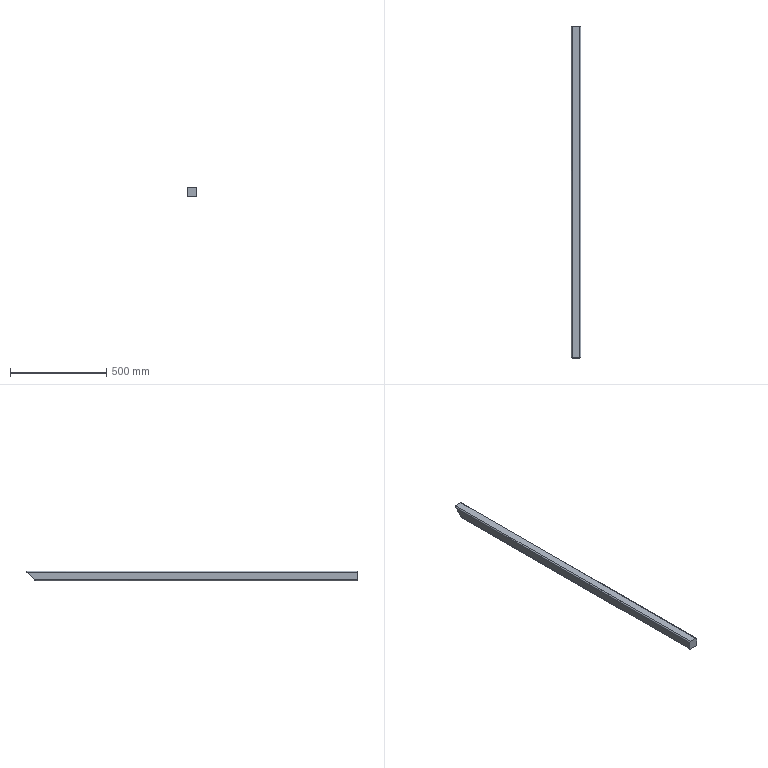Part | SolidWorks | features ICE 4, Extrusion 1 | 1 solid | 19 faces | box 50 x 1725 x 50 mm | volume 1494916 mm3 | plane 11 | cylinder 8 | commonest cylinder face diameters 2 x4 12 x4
STEP:
#1=CARTESIAN_POINT('',(-19.,1770.,7.278));
#2=VERTEX_POINT('',#1);
#3=CARTESIAN_POINT('',(-19.,60.,7.278));
#4=VERTEX_POINT('',#3);
#5=CARTESIAN_POINT('',(-19.,1775.,7.278));
#6=DIRECTION('',(0.,-1.,0.));
#7=VECTOR('',#6,1000.);
#8=LINE('',#5,#7);
#9=EDGE_CURVE('',#2,#4,#8,.T.);
#10=ORIENTED_EDGE('',*,*,#9,.T.);
#11=CARTESIAN_POINT('',(-20.,60.,6.278));
#12=VERTEX_POINT('',#11);
#13=CARTESIAN_POINT('',(-19.,60.,6.278));
#14=DIRECTION('',(0.,-1.,0.));
#15=DIRECTION('',(0.,0.,-1.));
#16=AXIS2_PLACEMENT_3D('',#13,#14,#15);
#17=CIRCLE('',#16,1.);
#18=EDGE_CURVE('',#4,#12,#17,.T.);
#19=ORIENTED_EDGE('',*,*,#18,.T.);
#20=CARTESIAN_POINT('',(-20.,1769.,6.278));
#21=VERTEX_POINT('',#20);
#22=CARTESIAN_POINT('',(-20.,1775.,6.278));
#23=DIRECTION('',(0.,-1.,0.));
#24=VECTOR('',#23,1000.);
#25=LINE('',#22,#24);
#26=EDGE_CURVE('',#21,#12,#25,.T.);
#27=ORIENTED_EDGE('',*,*,#26,.F.);
#28=CARTESIAN_POINT('',(-19.,1770.,7.278));
#29=CARTESIAN_POINT('',(-19.586,1770.,7.278));
#30=CARTESIAN_POINT('',(-20.,1769.586,6.864));
#31=CARTESIAN_POINT('',(-20.,1769.,6.278));
#32=(BOUNDED_CURVE()B_SPLINE_CURVE(3,(#28,#29,#30,#31),.UNSPECIFIED.,.F.,.F.)B_SPLINE_CURVE_WITH_KNOTS((4,4),(3.142,4.712),.UNSPECIFIED.)CURVE()GEOMETRIC_REPRESENTATION_ITEM()RATIONAL_B_SPLINE_CURVE((1.,0.8047,0.8047,1.))REPRESENTATION_ITEM(''));
#33=EDGE_CURVE('',#2,#21,#32,.T.);
#34=ORIENTED_EDGE('',*,*,#33,.F.);
#35=EDGE_LOOP('',(#10,#19,#27,#34));
#36=FACE_OUTER_BOUND('',#35,.T.);
#37=CARTESIAN_POINT('',(-19.,1775.,6.278));
#38=DIRECTION('',(0.,-1.,0.));
#39=DIRECTION('',(0.,0.,-1.));
#40=AXIS2_PLACEMENT_3D('',#37,#38,#39);
#41=CYLINDRICAL_SURFACE('',#40,1.);
#42=ADVANCED_FACE('',(#36),#41,.F.);
#43=CARTESIAN_POINT('',(19.,1770.,7.278));
#44=VERTEX_POINT('',#43);
#45=CARTESIAN_POINT('',(19.,60.,7.278));
#46=VERTEX_POINT('',#45);
#47=CARTESIAN_POINT('',(19.,1775.,7.278));
#48=DIRECTION('',(0.,-1.,0.));
#49=VECTOR('',#48,1000.);
#50=LINE('',#47,#49);
#51=EDGE_CURVE('',#44,#46,#50,.T.);
#52=ORIENTED_EDGE('',*,*,#51,.T.);
#53=CARTESIAN_POINT('',(-19.,60.,7.278));
#54=DIRECTION('',(-1.,0.,0.));
#55=VECTOR('',#54,1000.);
#56=LINE('',#53,#55);
#57=EDGE_CURVE('',#46,#4,#56,.T.);
#58=ORIENTED_EDGE('',*,*,#57,.T.);
#59=ORIENTED_EDGE('',*,*,#9,.F.);
#60=CARTESIAN_POINT('',(-19.,1770.,7.278));
#61=DIRECTION('',(-1.,0.,0.));
#62=VECTOR('',#61,1000.);
#63=LINE('',#60,#62);
#64=EDGE_CURVE('',#44,#2,#63,.T.);
#65=ORIENTED_EDGE('',*,*,#64,.F.);
#66=EDGE_LOOP('',(#52,#58,#59,#65));
#67=FACE_OUTER_BOUND('',#66,.T.);
#68=CARTESIAN_POINT('',(-19.,1775.,7.278));
#69=DIRECTION('',(0.,0.,-1.));
#70=DIRECTION('',(-1.,0.,0.));
#71=AXIS2_PLACEMENT_3D('',#68,#69,#70);
#72=PLANE('',#71);
#73=ADVANCED_FACE('',(#67),#72,.T.);
#74=CARTESIAN_POINT('',(20.,1769.,6.278));
#75=VERTEX_POINT('',#74);
#76=CARTESIAN_POINT('',(20.,60.,6.278));
#77=VERTEX_POINT('',#76);
#78=CARTESIAN_POINT('',(20.,1775.,6.278));
#79=DIRECTION('',(0.,-1.,0.));
#80=VECTOR('',#79,1000.);
#81=LINE('',#78,#80);
#82=EDGE_CURVE('',#75,#77,#81,.T.);
#83=ORIENTED_EDGE('',*,*,#82,.T.);
#84=CARTESIAN_POINT('',(19.,60.,6.278));
#85=DIRECTION('',(0.,-1.,0.));
#86=DIRECTION('',(0.,0.,-1.));
#87=AXIS2_PLACEMENT_3D('',#84,#85,#86);
#88=CIRCLE('',#87,1.);
#89=EDGE_CURVE('',#77,#46,#88,.T.);
#90=ORIENTED_EDGE('',*,*,#89,.T.);
#91=ORIENTED_EDGE('',*,*,#51,.F.);
#92=CARTESIAN_POINT('',(20.,1769.,6.278));
#93=CARTESIAN_POINT('',(20.,1769.586,6.864));
#94=CARTESIAN_POINT('',(19.586,1770.,7.278));
#95=CARTESIAN_POINT('',(19.,1770.,7.278));
#96=(BOUNDED_CURVE()B_SPLINE_CURVE(3,(#92,#93,#94,#95),.UNSPECIFIED.,.F.,.F.)B_SPLINE_CURVE_WITH_KNOTS((4,4),(1.571,3.142),.UNSPECIFIED.)CURVE()GEOMETRIC_REPRESENTATION_ITEM()RATIONAL_B_SPLINE_CURVE((1.,0.8047,0.8047,1.))REPRESENTATION_ITEM(''));
#97=EDGE_CURVE('',#75,#44,#96,.T.);
#98=ORIENTED_EDGE('',*,*,#97,.F.);
#99=EDGE_LOOP('',(#83,#90,#91,#98));
#100=FACE_OUTER_BOUND('',#99,.T.);
#101=CARTESIAN_POINT('',(19.,1775.,6.278));
#102=DIRECTION('',(0.,-1.,0.));
#103=DIRECTION('',(0.,0.,-1.));
#104=AXIS2_PLACEMENT_3D('',#101,#102,#103);
#105=CYLINDRICAL_SURFACE('',#104,1.);
#106=ADVANCED_FACE('',(#100),#105,.F.);
#107=CARTESIAN_POINT('',(20.,1731.,-31.722));
#108=VERTEX_POINT('',#107);
#109=CARTESIAN_POINT('',(20.,60.,-31.722));
#110=VERTEX_POINT('',#109);
#111=CARTESIAN_POINT('',(20.,1775.,-31.722));
#112=DIRECTION('',(0.,-1.,0.));
#113=VECTOR('',#112,1000.);
#114=LINE('',#111,#113);
#115=EDGE_CURVE('',#108,#110,#114,.T.);
#116=ORIENTED_EDGE('',*,*,#115,.T.);
#117=CARTESIAN_POINT('',(20.,60.,6.278));
#118=DIRECTION('',(0.,0.,1.));
#119=VECTOR('',#118,1000.);
#120=LINE('',#117,#119);
#121=EDGE_CURVE('',#110,#77,#120,.T.);
#122=ORIENTED_EDGE('',*,*,#121,.T.);
#123=ORIENTED_EDGE('',*,*,#82,.F.);
#124=CARTESIAN_POINT('',(20.,1772.,9.278));
#125=DIRECTION('',(0.,0.7071,0.7071));
#126=VECTOR('',#125,1000.);
#127=LINE('',#124,#126);
#128=EDGE_CURVE('',#108,#75,#127,.T.);
#129=ORIENTED_EDGE('',*,*,#128,.F.);
#130=EDGE_LOOP('',(#116,#122,#123,#129));
#131=FACE_OUTER_BOUND('',#130,.T.);
#132=CARTESIAN_POINT('',(20.,1775.,6.278));
#133=DIRECTION('',(-1.,0.,0.));
#134=DIRECTION('',(0.,0.,1.));
#135=AXIS2_PLACEMENT_3D('',#132,#133,#134);
#136=PLANE('',#135);
#137=ADVANCED_FACE('',(#131),#136,.T.);
#138=CARTESIAN_POINT('',(19.,1730.,-32.722));
#139=VERTEX_POINT('',#138);
#140=CARTESIAN_POINT('',(19.,60.,-32.722));
#141=VERTEX_POINT('',#140);
#142=CARTESIAN_POINT('',(19.,1775.,-32.722));
#143=DIRECTION('',(0.,-1.,0.));
#144=VECTOR('',#143,1000.);
#145=LINE('',#142,#144);
#146=EDGE_CURVE('',#139,#141,#145,.T.);
#147=ORIENTED_EDGE('',*,*,#146,.T.);
#148=CARTESIAN_POINT('',(19.,60.,-31.722));
#149=DIRECTION('',(0.,-1.,0.));
#150=DIRECTION('',(0.,0.,-1.));
#151=AXIS2_PLACEMENT_3D('',#148,#149,#150);
#152=CIRCLE('',#151,1.);
#153=EDGE_CURVE('',#141,#110,#152,.T.);
#154=ORIENTED_EDGE('',*,*,#153,.T.);
#155=ORIENTED_EDGE('',*,*,#115,.F.);
#156=CARTESIAN_POINT('',(19.,1730.,-32.722));
#157=CARTESIAN_POINT('',(19.586,1730.,-32.722));
#158=CARTESIAN_POINT('',(20.,1730.414,-32.308));
#159=CARTESIAN_POINT('',(20.,1731.,-31.722));
#160=(BOUNDED_CURVE()B_SPLINE_CURVE(3,(#156,#157,#158,#159),.UNSPECIFIED.,.F.,.F.)B_SPLINE_CURVE_WITH_KNOTS((4,4),(0.,1.571),.UNSPECIFIED.)CURVE()GEOMETRIC_REPRESENTATION_ITEM()RATIONAL_B_SPLINE_CURVE((1.,0.8047,0.8047,1.))REPRESENTATION_ITEM(''));
#161=EDGE_CURVE('',#139,#108,#160,.T.);
#162=ORIENTED_EDGE('',*,*,#161,.F.);
#163=EDGE_LOOP('',(#147,#154,#155,#162));
#164=FACE_OUTER_BOUND('',#163,.T.);
#165=CARTESIAN_POINT('',(19.,1775.,-31.722));
#166=DIRECTION('',(0.,-1.,0.));
#167=DIRECTION('',(0.,0.,-1.));
#168=AXIS2_PLACEMENT_3D('',#165,#166,#167);
#169=CYLINDRICAL_SURFACE('',#168,1.);
#170=ADVANCED_FACE('',(#164),#169,.F.);
#171=CARTESIAN_POINT('',(-19.,1730.,-32.722));
#172=VERTEX_POINT('',#171);
#173=CARTESIAN_POINT('',(-19.,60.,-32.722));
#174=VERTEX_POINT('',#173);
#175=CARTESIAN_POINT('',(-19.,1775.,-32.722));
#176=DIRECTION('',(0.,-1.,0.));
#177=VECTOR('',#176,1000.);
#178=LINE('',#175,#177);
#179=EDGE_CURVE('',#172,#174,#178,.T.);
#180=ORIENTED_EDGE('',*,*,#179,.T.);
#181=CARTESIAN_POINT('',(-19.,60.,-32.722));
#182=DIRECTION('',(1.,0.,0.));
#183=VECTOR('',#182,1000.);
#184=LINE('',#181,#183);
#185=EDGE_CURVE('',#174,#141,#184,.T.);
#186=ORIENTED_EDGE('',*,*,#185,.T.);
#187=ORIENTED_EDGE('',*,*,#146,.F.);
#188=CARTESIAN_POINT('',(-19.,1730.,-32.722));
#189=DIRECTION('',(1.,0.,0.));
#190=VECTOR('',#189,1000.);
#191=LINE('',#188,#190);
#192=EDGE_CURVE('',#172,#139,#191,.T.);
#193=ORIENTED_EDGE('',*,*,#192,.F.);
#194=EDGE_LOOP('',(#180,#186,#187,#193));
#195=FACE_OUTER_BOUND('',#194,.T.);
#196=CARTESIAN_POINT('',(-19.,1775.,-32.722));
#197=DIRECTION('',(0.,0.,1.));
#198=DIRECTION('',(1.,0.,0.));
#199=AXIS2_PLACEMENT_3D('',#196,#197,#198);
#200=PLANE('',#199);
#201=ADVANCED_FACE('',(#195),#200,.T.);
#202=CARTESIAN_POINT('',(-20.,1731.,-31.722));
#203=VERTEX_POINT('',#202);
#204=CARTESIAN_POINT('',(-20.,60.,-31.722));
#205=VERTEX_POINT('',#204);
#206=CARTESIAN_POINT('',(-20.,1775.,-31.722));
#207=DIRECTION('',(0.,-1.,0.));
#208=VECTOR('',#207,1000.);
#209=LINE('',#206,#208);
#210=EDGE_CURVE('',#203,#205,#209,.T.);
#211=ORIENTED_EDGE('',*,*,#210,.T.);
#212=CARTESIAN_POINT('',(-19.,60.,-31.722));
#213=DIRECTION('',(0.,-1.,0.));
#214=DIRECTION('',(0.,0.,-1.));
#215=AXIS2_PLACEMENT_3D('',#212,#213,#214);
#216=CIRCLE('',#215,1.);
#217=EDGE_CURVE('',#205,#174,#216,.T.);
#218=ORIENTED_EDGE('',*,*,#217,.T.);
#219=ORIENTED_EDGE('',*,*,#179,.F.);
#220=CARTESIAN_POINT('',(-20.,1731.,-31.722));
#221=CARTESIAN_POINT('',(-20.,1730.414,-32.308));
#222=CARTESIAN_POINT('',(-19.586,1730.,-32.722));
#223=CARTESIAN_POINT('',(-19.,1730.,-32.722));
#224=(BOUNDED_CURVE()B_SPLINE_CURVE(3,(#220,#221,#222,#223),.UNSPECIFIED.,.F.,.F.)B_SPLINE_CURVE_WITH_KNOTS((4,4),(4.712,6.283),.UNSPECIFIED.)CURVE()GEOMETRIC_REPRESENTATION_ITEM()RATIONAL_B_SPLINE_CURVE((1.,0.8047,0.8047,1.))REPRESENTATION_ITEM(''));
#225=EDGE_CURVE('',#203,#172,#224,.T.);
#226=ORIENTED_EDGE('',*,*,#225,.F.);
#227=EDGE_LOOP('',(#211,#218,#219,#226));
#228=FACE_OUTER_BOUND('',#227,.T.);
#229=CARTESIAN_POINT('',(-19.,1775.,-31.722));
#230=DIRECTION('',(0.,-1.,0.));
#231=DIRECTION('',(0.,0.,-1.));
#232=AXIS2_PLACEMENT_3D('',#229,#230,#231);
#233=CYLINDRICAL_SURFACE('',#232,1.);
#234=ADVANCED_FACE('',(#228),#233,.F.);
#235=ORIENTED_EDGE('',*,*,#26,.T.);
#236=CARTESIAN_POINT('',(-20.,60.,6.278));
#237=DIRECTION('',(0.,0.,-1.));
#238=VECTOR('',#237,1000.);
#239=LINE('',#236,#238);
#240=EDGE_CURVE('',#12,#205,#239,.T.);
#241=ORIENTED_EDGE('',*,*,#240,.T.);
#242=ORIENTED_EDGE('',*,*,#210,.F.);
#243=CARTESIAN_POINT('',(-20.,1772.,9.278));
#244=DIRECTION('',(0.,-0.7071,-0.7071));
#245=VECTOR('',#244,1000.);
#246=LINE('',#243,#245);
#247=EDGE_CURVE('',#21,#203,#246,.T.);
#248=ORIENTED_EDGE('',*,*,#247,.F.);
#249=EDGE_LOOP('',(#235,#241,#242,#248));
#250=FACE_OUTER_BOUND('',#249,.T.);
#251=CARTESIAN_POINT('',(-20.,1775.,6.278));
#252=DIRECTION('',(1.,0.,0.));
#253=DIRECTION('',(0.,0.,-1.));
#254=AXIS2_PLACEMENT_3D('',#251,#252,#253);
#255=PLANE('',#254);
#256=ADVANCED_FACE('',(#250),#255,.T.);
#257=CARTESIAN_POINT('',(-25.,50.,6.278));
#258=VERTEX_POINT('',#257);
#259=CARTESIAN_POINT('',(-19.,50.,12.278));
#260=VERTEX_POINT('',#259);
#261=CARTESIAN_POINT('',(-19.,50.,6.278));
#262=DIRECTION('',(0.,1.,0.));
#263=DIRECTION('',(0.,0.,1.));
#264=AXIS2_PLACEMENT_3D('',#261,#262,#263);
#265=CIRCLE('',#264,6.);
#266=EDGE_CURVE('',#258,#260,#265,.T.);
#267=ORIENTED_EDGE('',*,*,#266,.T.);
#268=CARTESIAN_POINT('',(-19.,1775.,12.278));
#269=VERTEX_POINT('',#268);
#270=CARTESIAN_POINT('',(-19.,1775.,12.278));
#271=DIRECTION('',(0.,-1.,0.));
#272=VECTOR('',#271,1000.);
#273=LINE('',#270,#272);
#274=EDGE_CURVE('',#269,#260,#273,.T.);
#275=ORIENTED_EDGE('',*,*,#274,.F.);
#276=CARTESIAN_POINT('',(-25.,1769.,6.278));
#277=VERTEX_POINT('',#276);
#278=CARTESIAN_POINT('',(-19.,1775.,12.278));
#279=CARTESIAN_POINT('',(-22.515,1775.,12.278));
#280=CARTESIAN_POINT('',(-25.,1772.515,9.793));
#281=CARTESIAN_POINT('',(-25.,1769.,6.278));
#282=(BOUNDED_CURVE()B_SPLINE_CURVE(3,(#278,#279,#280,#281),.UNSPECIFIED.,.F.,.F.)B_SPLINE_CURVE_WITH_KNOTS((4,4),(3.142,4.712),.UNSPECIFIED.)CURVE()GEOMETRIC_REPRESENTATION_ITEM()RATIONAL_B_SPLINE_CURVE((1.,0.8047,0.8047,1.))REPRESENTATION_ITEM(''));
#283=EDGE_CURVE('',#269,#277,#282,.T.);
#284=ORIENTED_EDGE('',*,*,#283,.T.);
#285=CARTESIAN_POINT('',(-25.,1775.,6.278));
#286=DIRECTION('',(0.,-1.,0.));
#287=VECTOR('',#286,1000.);
#288=LINE('',#285,#287);
#289=EDGE_CURVE('',#277,#258,#288,.T.);
#290=ORIENTED_EDGE('',*,*,#289,.T.);
#291=EDGE_LOOP('',(#267,#275,#284,#290));
#292=FACE_OUTER_BOUND('',#291,.T.);
#293=CARTESIAN_POINT('',(-19.,1775.,6.278));
#294=DIRECTION('',(0.,-1.,0.));
#295=DIRECTION('',(0.,0.,-1.));
#296=AXIS2_PLACEMENT_3D('',#293,#294,#295);
#297=CYLINDRICAL_SURFACE('',#296,6.);
#298=ADVANCED_FACE('',(#292),#297,.T.);
#299=CARTESIAN_POINT('',(19.,50.,12.278));
#300=VERTEX_POINT('',#299);
#301=CARTESIAN_POINT('',(-19.,50.,12.278));
#302=DIRECTION('',(1.,0.,0.));
#303=VECTOR('',#302,1000.);
#304=LINE('',#301,#303);
#305=EDGE_CURVE('',#260,#300,#304,.T.);
#306=ORIENTED_EDGE('',*,*,#305,.T.);
#307=CARTESIAN_POINT('',(19.,1775.,12.278));
#308=VERTEX_POINT('',#307);
#309=CARTESIAN_POINT('',(19.,1775.,12.278));
#310=DIRECTION('',(0.,-1.,0.));
#311=VECTOR('',#310,1000.);
#312=LINE('',#309,#311);
#313=EDGE_CURVE('',#308,#300,#312,.T.);
#314=ORIENTED_EDGE('',*,*,#313,.F.);
#315=CARTESIAN_POINT('',(-19.,1775.,12.278));
#316=DIRECTION('',(1.,0.,0.));
#317=VECTOR('',#316,1000.);
#318=LINE('',#315,#317);
#319=EDGE_CURVE('',#269,#308,#318,.T.);
#320=ORIENTED_EDGE('',*,*,#319,.F.);
#321=ORIENTED_EDGE('',*,*,#274,.T.);
#322=EDGE_LOOP('',(#306,#314,#320,#321));
#323=FACE_OUTER_BOUND('',#322,.T.);
#324=CARTESIAN_POINT('',(-19.,1775.,12.278));
#325=DIRECTION('',(0.,0.,-1.));
#326=DIRECTION('',(-1.,0.,0.));
#327=AXIS2_PLACEMENT_3D('',#324,#325,#326);
#328=PLANE('',#327);
#329=ADVANCED_FACE('',(#323),#328,.F.);
#330=CARTESIAN_POINT('',(25.,50.,6.278));
#331=VERTEX_POINT('',#330);
#332=CARTESIAN_POINT('',(19.,50.,6.278));
#333=DIRECTION('',(0.,1.,0.));
#334=DIRECTION('',(0.,0.,1.));
#335=AXIS2_PLACEMENT_3D('',#332,#333,#334);
#336=CIRCLE('',#335,6.);
#337=EDGE_CURVE('',#300,#331,#336,.T.);
#338=ORIENTED_EDGE('',*,*,#337,.T.);
#339=CARTESIAN_POINT('',(25.,1769.,6.278));
#340=VERTEX_POINT('',#339);
#341=CARTESIAN_POINT('',(25.,1775.,6.278));
#342=DIRECTION('',(0.,-1.,0.));
#343=VECTOR('',#342,1000.);
#344=LINE('',#341,#343);
#345=EDGE_CURVE('',#340,#331,#344,.T.);
#346=ORIENTED_EDGE('',*,*,#345,.F.);
#347=CARTESIAN_POINT('',(25.,1769.,6.278));
#348=CARTESIAN_POINT('',(25.,1772.515,9.793));
#349=CARTESIAN_POINT('',(22.515,1775.,12.278));
#350=CARTESIAN_POINT('',(19.,1775.,12.278));
#351=(BOUNDED_CURVE()B_SPLINE_CURVE(3,(#347,#348,#349,#350),.UNSPECIFIED.,.F.,.F.)B_SPLINE_CURVE_WITH_KNOTS((4,4),(1.571,3.142),.UNSPECIFIED.)CURVE()GEOMETRIC_REPRESENTATION_ITEM()RATIONAL_B_SPLINE_CURVE((1.,0.8047,0.8047,1.))REPRESENTATION_ITEM(''));
#352=EDGE_CURVE('',#340,#308,#351,.T.);
#353=ORIENTED_EDGE('',*,*,#352,.T.);
#354=ORIENTED_EDGE('',*,*,#313,.T.);
#355=EDGE_LOOP('',(#338,#346,#353,#354));
#356=FACE_OUTER_BOUND('',#355,.T.);
#357=CARTESIAN_POINT('',(19.,1775.,6.278));
#358=DIRECTION('',(0.,-1.,0.));
#359=DIRECTION('',(0.,0.,-1.));
#360=AXIS2_PLACEMENT_3D('',#357,#358,#359);
#361=CYLINDRICAL_SURFACE('',#360,6.);
#362=ADVANCED_FACE('',(#356),#361,.T.);
#363=CARTESIAN_POINT('',(25.,50.,-31.722));
#364=VERTEX_POINT('',#363);
#365=CARTESIAN_POINT('',(25.,50.,341.265));
#366=DIRECTION('',(0.,0.,1.));
#367=VECTOR('',#366,1000.);
#368=LINE('',#365,#367);
#369=EDGE_CURVE('',#364,#331,#368,.T.);
#370=ORIENTED_EDGE('',*,*,#369,.F.);
#371=CARTESIAN_POINT('',(25.,1731.,-31.722));
#372=VERTEX_POINT('',#371);
#373=CARTESIAN_POINT('',(25.,1775.,-31.722));
#374=DIRECTION('',(0.,-1.,0.));
#375=VECTOR('',#374,1000.);
#376=LINE('',#373,#375);
#377=EDGE_CURVE('',#372,#364,#376,.T.);
#378=ORIENTED_EDGE('',*,*,#377,.F.);
#379=CARTESIAN_POINT('',(25.,1725.,-37.722));
#380=DIRECTION('',(0.,-0.7071,-0.7071));
#381=VECTOR('',#380,1000.);
#382=LINE('',#379,#381);
#383=EDGE_CURVE('',#340,#372,#382,.T.);
#384=ORIENTED_EDGE('',*,*,#383,.F.);
#385=ORIENTED_EDGE('',*,*,#345,.T.);
#386=EDGE_LOOP('',(#370,#378,#384,#385));
#387=FACE_OUTER_BOUND('',#386,.T.);
#388=CARTESIAN_POINT('',(25.,1775.,6.278));
#389=DIRECTION('',(-1.,0.,0.));
#390=DIRECTION('',(0.,0.,1.));
#391=AXIS2_PLACEMENT_3D('',#388,#389,#390);
#392=PLANE('',#391);
#393=ADVANCED_FACE('',(#387),#392,.F.);
#394=CARTESIAN_POINT('',(19.,50.,-37.722));
#395=VERTEX_POINT('',#394);
#396=CARTESIAN_POINT('',(19.,50.,-31.722));
#397=DIRECTION('',(0.,1.,0.));
#398=DIRECTION('',(0.,0.,1.));
#399=AXIS2_PLACEMENT_3D('',#396,#397,#398);
#400=CIRCLE('',#399,6.);
#401=EDGE_CURVE('',#364,#395,#400,.T.);
#402=ORIENTED_EDGE('',*,*,#401,.T.);
#403=CARTESIAN_POINT('',(19.,1725.,-37.722));
#404=VERTEX_POINT('',#403);
#405=CARTESIAN_POINT('',(19.,1775.,-37.722));
#406=DIRECTION('',(0.,-1.,0.));
#407=VECTOR('',#406,1000.);
#408=LINE('',#405,#407);
#409=EDGE_CURVE('',#404,#395,#408,.T.);
#410=ORIENTED_EDGE('',*,*,#409,.F.);
#411=CARTESIAN_POINT('',(19.,1725.,-37.722));
#412=CARTESIAN_POINT('',(22.515,1725.,-37.722));
#413=CARTESIAN_POINT('',(25.,1727.485,-35.237));
#414=CARTESIAN_POINT('',(25.,1731.,-31.722));
#415=(BOUNDED_CURVE()B_SPLINE_CURVE(3,(#411,#412,#413,#414),.UNSPECIFIED.,.F.,.F.)B_SPLINE_CURVE_WITH_KNOTS((4,4),(0.,1.571),.UNSPECIFIED.)CURVE()GEOMETRIC_REPRESENTATION_ITEM()RATIONAL_B_SPLINE_CURVE((1.,0.8047,0.8047,1.))REPRESENTATION_ITEM(''));
#416=EDGE_CURVE('',#404,#372,#415,.T.);
#417=ORIENTED_EDGE('',*,*,#416,.T.);
#418=ORIENTED_EDGE('',*,*,#377,.T.);
#419=EDGE_LOOP('',(#402,#410,#417,#418));
#420=FACE_OUTER_BOUND('',#419,.T.);
#421=CARTESIAN_POINT('',(19.,1775.,-31.722));
#422=DIRECTION('',(0.,-1.,0.));
#423=DIRECTION('',(0.,0.,-1.));
#424=AXIS2_PLACEMENT_3D('',#421,#422,#423);
#425=CYLINDRICAL_SURFACE('',#424,6.);
#426=ADVANCED_FACE('',(#420),#425,.T.);
#427=CARTESIAN_POINT('',(-19.,50.,-37.722));
#428=VERTEX_POINT('',#427);
#429=CARTESIAN_POINT('',(-19.,50.,-37.722));
#430=DIRECTION('',(-1.,0.,0.));
#431=VECTOR('',#430,1000.);
#432=LINE('',#429,#431);
#433=EDGE_CURVE('',#395,#428,#432,.T.);
#434=ORIENTED_EDGE('',*,*,#433,.T.);
#435=CARTESIAN_POINT('',(-19.,1725.,-37.722));
#436=VERTEX_POINT('',#435);
#437=CARTESIAN_POINT('',(-19.,1775.,-37.722));
#438=DIRECTION('',(0.,-1.,0.));
#439=VECTOR('',#438,1000.);
#440=LINE('',#437,#439);
#441=EDGE_CURVE('',#436,#428,#440,.T.);
#442=ORIENTED_EDGE('',*,*,#441,.F.);
#443=CARTESIAN_POINT('',(-25.,1725.,-37.722));
#444=DIRECTION('',(1.,0.,0.));
#445=VECTOR('',#444,1000.);
#446=LINE('',#443,#445);
#447=EDGE_CURVE('',#436,#404,#446,.T.);
#448=ORIENTED_EDGE('',*,*,#447,.T.);
#449=ORIENTED_EDGE('',*,*,#409,.T.);
#450=EDGE_LOOP('',(#434,#442,#448,#449));
#451=FACE_OUTER_BOUND('',#450,.T.);
#452=CARTESIAN_POINT('',(-19.,1775.,-37.722));
#453=DIRECTION('',(0.,0.,1.));
#454=DIRECTION('',(1.,0.,0.));
#455=AXIS2_PLACEMENT_3D('',#452,#453,#454);
#456=PLANE('',#455);
#457=ADVANCED_FACE('',(#451),#456,.F.);
#458=CARTESIAN_POINT('',(-25.,50.,-31.722));
#459=VERTEX_POINT('',#458);
#460=CARTESIAN_POINT('',(-19.,50.,-31.722));
#461=DIRECTION('',(0.,1.,0.));
#462=DIRECTION('',(0.,0.,1.));
#463=AXIS2_PLACEMENT_3D('',#460,#461,#462);
#464=CIRCLE('',#463,6.);
#465=EDGE_CURVE('',#428,#459,#464,.T.);
#466=ORIENTED_EDGE('',*,*,#465,.T.);
#467=CARTESIAN_POINT('',(-25.,1731.,-31.722));
#468=VERTEX_POINT('',#467);
#469=CARTESIAN_POINT('',(-25.,1775.,-31.722));
#470=DIRECTION('',(0.,-1.,0.));
#471=VECTOR('',#470,1000.);
#472=LINE('',#469,#471);
#473=EDGE_CURVE('',#468,#459,#472,.T.);
#474=ORIENTED_EDGE('',*,*,#473,.F.);
#475=CARTESIAN_POINT('',(-25.,1731.,-31.722));
#476=CARTESIAN_POINT('',(-25.,1727.485,-35.237));
#477=CARTESIAN_POINT('',(-22.515,1725.,-37.722));
#478=CARTESIAN_POINT('',(-19.,1725.,-37.722));
#479=(BOUNDED_CURVE()B_SPLINE_CURVE(3,(#475,#476,#477,#478),.UNSPECIFIED.,.F.,.F.)B_SPLINE_CURVE_WITH_KNOTS((4,4),(4.712,6.283),.UNSPECIFIED.)CURVE()GEOMETRIC_REPRESENTATION_ITEM()RATIONAL_B_SPLINE_CURVE((1.,0.8047,0.8047,1.))REPRESENTATION_ITEM(''));
#480=EDGE_CURVE('',#468,#436,#479,.T.);
#481=ORIENTED_EDGE('',*,*,#480,.T.);
#482=ORIENTED_EDGE('',*,*,#441,.T.);
#483=EDGE_LOOP('',(#466,#474,#481,#482));
#484=FACE_OUTER_BOUND('',#483,.T.);
#485=CARTESIAN_POINT('',(-19.,1775.,-31.722));
#486=DIRECTION('',(0.,-1.,0.));
#487=DIRECTION('',(0.,0.,-1.));
#488=AXIS2_PLACEMENT_3D('',#485,#486,#487);
#489=CYLINDRICAL_SURFACE('',#488,6.);
#490=ADVANCED_FACE('',(#484),#489,.T.);
#491=CARTESIAN_POINT('',(-25.,50.,6.278));
#492=DIRECTION('',(0.,0.,1.));
#493=VECTOR('',#492,1000.);
#494=LINE('',#491,#493);
#495=EDGE_CURVE('',#459,#258,#494,.T.);
#496=ORIENTED_EDGE('',*,*,#495,.T.);
#497=ORIENTED_EDGE('',*,*,#289,.F.);
#498=CARTESIAN_POINT('',(-25.,1725.,-37.722));
#499=DIRECTION('',(0.,-0.7071,-0.7071));
#500=VECTOR('',#499,1000.);
#501=LINE('',#498,#500);
#502=EDGE_CURVE('',#277,#468,#501,.T.);
#503=ORIENTED_EDGE('',*,*,#502,.T.);
#504=ORIENTED_EDGE('',*,*,#473,.T.);
#505=EDGE_LOOP('',(#496,#497,#503,#504));
#506=FACE_OUTER_BOUND('',#505,.T.);
#507=CARTESIAN_POINT('',(-25.,1775.,6.278));
#508=DIRECTION('',(1.,0.,0.));
#509=DIRECTION('',(0.,0.,-1.));
#510=AXIS2_PLACEMENT_3D('',#507,#508,#509);
#511=PLANE('',#510);
#512=ADVANCED_FACE('',(#506),#511,.F.);
#513=ORIENTED_EDGE('',*,*,#33,.T.);
#514=ORIENTED_EDGE('',*,*,#247,.T.);
#515=ORIENTED_EDGE('',*,*,#225,.T.);
#516=ORIENTED_EDGE('',*,*,#192,.T.);
#517=ORIENTED_EDGE('',*,*,#161,.T.);
#518=ORIENTED_EDGE('',*,*,#128,.T.);
#519=ORIENTED_EDGE('',*,*,#97,.T.);
#520=ORIENTED_EDGE('',*,*,#64,.T.);
#521=EDGE_LOOP('',(#513,#514,#515,#516,#517,#518,#519,#520));
#522=FACE_BOUND('',#521,.T.);
#523=ORIENTED_EDGE('',*,*,#319,.T.);
#524=ORIENTED_EDGE('',*,*,#352,.F.);
#525=ORIENTED_EDGE('',*,*,#383,.T.);
#526=ORIENTED_EDGE('',*,*,#416,.F.);
#527=ORIENTED_EDGE('',*,*,#447,.F.);
#528=ORIENTED_EDGE('',*,*,#480,.F.);
#529=ORIENTED_EDGE('',*,*,#502,.F.);
#530=ORIENTED_EDGE('',*,*,#283,.F.);
#531=EDGE_LOOP('',(#523,#524,#525,#526,#527,#528,#529,#530));
#532=FACE_OUTER_BOUND('',#531,.T.);
#533=CARTESIAN_POINT('',(-25.,1725.,-37.722));
#534=DIRECTION('',(0.,-0.7071,0.7071));
#535=DIRECTION('',(0.,-0.7071,-0.7071));
#536=AXIS2_PLACEMENT_3D('',#533,#534,#535);
#537=PLANE('',#536);
#538=ADVANCED_FACE('',(#522,#532),#537,.F.);
#539=ORIENTED_EDGE('',*,*,#495,.F.);
#540=ORIENTED_EDGE('',*,*,#465,.F.);
#541=ORIENTED_EDGE('',*,*,#433,.F.);
#542=ORIENTED_EDGE('',*,*,#401,.F.);
#543=ORIENTED_EDGE('',*,*,#369,.T.);
#544=ORIENTED_EDGE('',*,*,#337,.F.);
#545=ORIENTED_EDGE('',*,*,#305,.F.);
#546=ORIENTED_EDGE('',*,*,#266,.F.);
#547=EDGE_LOOP('',(#539,#540,#541,#542,#543,#544,#545,#546));
#548=FACE_OUTER_BOUND('',#547,.T.);
#549=CARTESIAN_POINT('',(-25.,50.,341.265));
#550=DIRECTION('',(0.,1.,0.));
#551=DIRECTION('',(0.,0.,1.));
#552=AXIS2_PLACEMENT_3D('',#549,#550,#551);
#553=PLANE('',#552);
#554=ADVANCED_FACE('',(#548),#553,.F.);
#555=ORIENTED_EDGE('',*,*,#18,.F.);
#556=ORIENTED_EDGE('',*,*,#57,.F.);
#557=ORIENTED_EDGE('',*,*,#89,.F.);
#558=ORIENTED_EDGE('',*,*,#121,.F.);
#559=ORIENTED_EDGE('',*,*,#153,.F.);
#560=ORIENTED_EDGE('',*,*,#185,.F.);
#561=ORIENTED_EDGE('',*,*,#217,.F.);
#562=ORIENTED_EDGE('',*,*,#240,.F.);
#563=EDGE_LOOP('',(#555,#556,#557,#558,#559,#560,#561,#562));
#564=FACE_OUTER_BOUND('',#563,.T.);
#565=CARTESIAN_POINT('',(-19.,60.,6.278));
#566=DIRECTION('',(0.,-1.,0.));
#567=DIRECTION('',(0.,0.,-1.));
#568=AXIS2_PLACEMENT_3D('',#565,#566,#567);
#569=PLANE('',#568);
#570=ADVANCED_FACE('',(#564),#569,.F.);
#571=CLOSED_SHELL('',(#42,#73,#106,#137,#170,#201,#234,#256,#298,#329,#362,#393,#426,#457,#490,#512,#538,#554,#570));
#572=MANIFOLD_SOLID_BREP('',#571);
#573=CARTESIAN_POINT('',(0.,0.,0.));
#574=DIRECTION('',(0.,0.,1.));
#575=DIRECTION('',(1.,0.,0.));
#576=AXIS2_PLACEMENT_3D('',#573,#574,#575);
#577=(LENGTH_UNIT()NAMED_UNIT(*)SI_UNIT(.MILLI.,.METRE.));
#578=UNCERTAINTY_MEASURE_WITH_UNIT(LENGTH_MEASURE(0.00001),#577,'','');
#579=(NAMED_UNIT(*)PLANE_ANGLE_UNIT()SI_UNIT($,.RADIAN.));
#580=(NAMED_UNIT(*)SI_UNIT($,.STERADIAN.)SOLID_ANGLE_UNIT());
#581=(GEOMETRIC_REPRESENTATION_CONTEXT(3)GLOBAL_UNCERTAINTY_ASSIGNED_CONTEXT((#578))GLOBAL_UNIT_ASSIGNED_CONTEXT((#577,#579,#580))REPRESENTATION_CONTEXT('',''));
#582=ADVANCED_BREP_SHAPE_REPRESENTATION('',(#572,#576),#581);